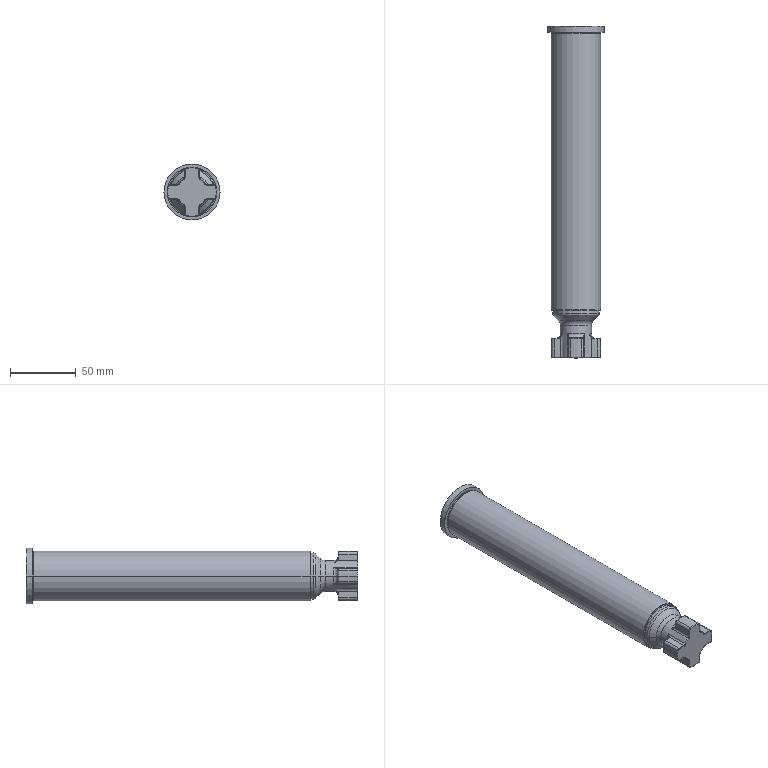Part | SolidWorks | features BaseBody 1, Scale 1 | 1 solid | 135 faces | box 42.588 x 252.216 x 42.588 mm | volume 265706 mm3 | torus 53 | cylinder 47 | plane 17 | spline 16 | cone 2 | commonest cylinder face diameters 0.946 x16 3.786 x16 37.619 x7 23.66 x2 35.253 x2 36.2 x2